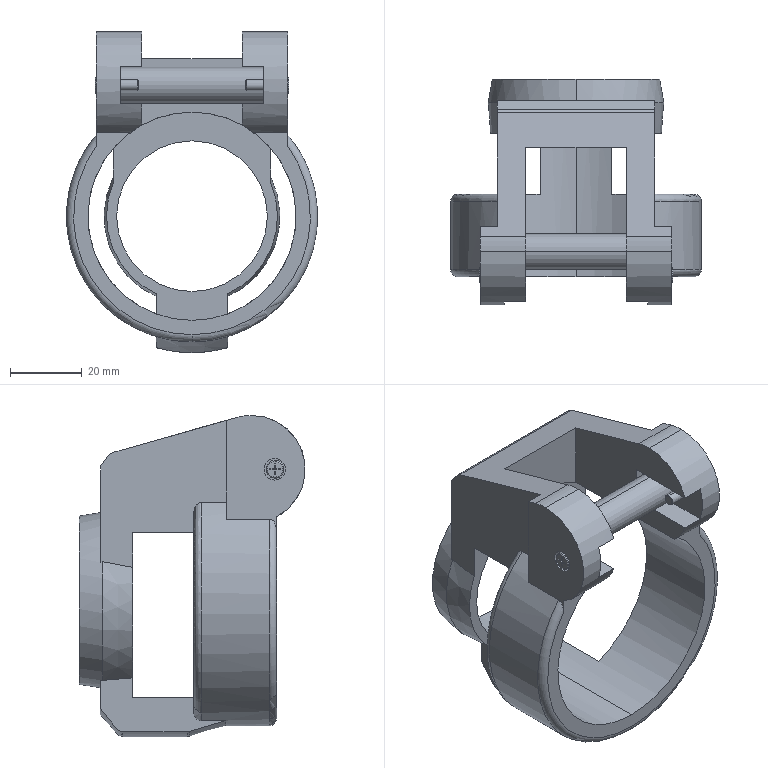Part | STEP file | _CGR51-60-U-002.stp | 1 solid | 130 faces | box 70 x 63 x 89.5 mm | volume 67213 mm3 | plane 62 | cone 31 | cylinder 29 | torus 8 | commonest cylinder face diameters 3 x6 5 x4 6 x4 30 x4 10 x2 42 x2